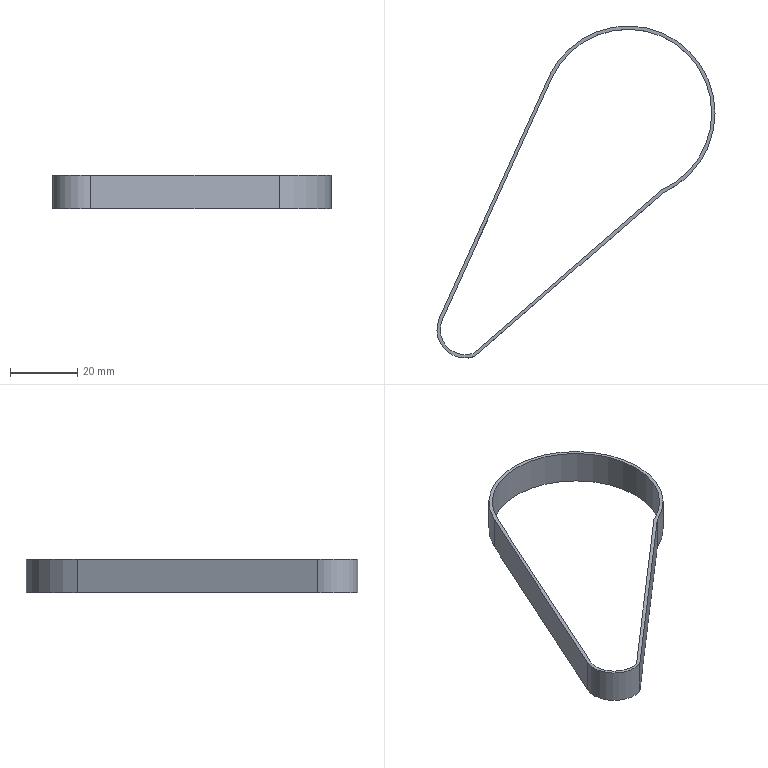Part | SolidWorks | features ExtruThin 1 | 1 solid | 12 faces | box 83.007 x 99.109 x 10 mm | volume 2707 mm3 | cylinder 6 | plane 6 | commonest cylinder face diameters 50 x2 52 x2 15 x1 17 x1
STEP:
#1=CARTESIAN_POINT('',(13.626,44.609,-10.));
#2=VERTEX_POINT('',#1);
#3=CARTESIAN_POINT('',(-34.143,54.932,-10.));
#4=VERTEX_POINT('',#3);
#5=CARTESIAN_POINT('',(-11.374,44.609,-10.));
#6=DIRECTION('',(0.,0.,1.));
#7=DIRECTION('',(1.,0.,0.));
#8=AXIS2_PLACEMENT_3D('',#5,#6,#7);
#9=CIRCLE('',#8,25.);
#10=EDGE_CURVE('',#2,#4,#9,.T.);
#11=ORIENTED_EDGE('',*,*,#10,.F.);
#12=CARTESIAN_POINT('',(13.626,44.609,0.));
#13=VERTEX_POINT('',#12);
#14=CARTESIAN_POINT('',(13.626,44.609,-10.));
#15=DIRECTION('',(0.,0.,1.));
#16=VECTOR('',#15,1000.);
#17=LINE('',#14,#16);
#18=EDGE_CURVE('',#2,#13,#17,.T.);
#19=ORIENTED_EDGE('',*,*,#18,.T.);
#20=CARTESIAN_POINT('',(-34.143,54.932,0.));
#21=VERTEX_POINT('',#20);
#22=CARTESIAN_POINT('',(-11.374,44.609,0.));
#23=DIRECTION('',(0.,0.,1.));
#24=DIRECTION('',(1.,0.,0.));
#25=AXIS2_PLACEMENT_3D('',#22,#23,#24);
#26=CIRCLE('',#25,25.);
#27=EDGE_CURVE('',#13,#21,#26,.T.);
#28=ORIENTED_EDGE('',*,*,#27,.T.);
#29=CARTESIAN_POINT('',(-34.143,54.932,-10.));
#30=DIRECTION('',(0.,0.,1.));
#31=VECTOR('',#30,1000.);
#32=LINE('',#29,#31);
#33=EDGE_CURVE('',#4,#21,#32,.T.);
#34=ORIENTED_EDGE('',*,*,#33,.F.);
#35=EDGE_LOOP('',(#11,#19,#28,#34));
#36=FACE_OUTER_BOUND('',#35,.T.);
#37=CARTESIAN_POINT('',(-11.374,44.609,-10.));
#38=DIRECTION('',(0.,0.,1.));
#39=DIRECTION('',(1.,0.,0.));
#40=AXIS2_PLACEMENT_3D('',#37,#38,#39);
#41=CYLINDRICAL_SURFACE('',#40,25.);
#42=ADVANCED_FACE('',(#36),#41,.F.);
#43=CARTESIAN_POINT('',(-0.8671,20.826,-10.));
#44=VERTEX_POINT('',#43);
#45=CARTESIAN_POINT('',(14.626,44.609,-10.));
#46=VERTEX_POINT('',#45);
#47=CARTESIAN_POINT('',(-11.374,44.609,-10.));
#48=DIRECTION('',(0.,0.,1.));
#49=DIRECTION('',(1.,0.,0.));
#50=AXIS2_PLACEMENT_3D('',#47,#48,#49);
#51=CIRCLE('',#50,26.);
#52=EDGE_CURVE('',#44,#46,#51,.T.);
#53=ORIENTED_EDGE('',*,*,#52,.T.);
#54=CARTESIAN_POINT('',(14.626,44.609,0.));
#55=VERTEX_POINT('',#54);
#56=CARTESIAN_POINT('',(14.626,44.609,-10.));
#57=DIRECTION('',(0.,0.,1.));
#58=VECTOR('',#57,1000.);
#59=LINE('',#56,#58);
#60=EDGE_CURVE('',#46,#55,#59,.T.);
#61=ORIENTED_EDGE('',*,*,#60,.T.);
#62=CARTESIAN_POINT('',(-0.8671,20.826,0.));
#63=VERTEX_POINT('',#62);
#64=CARTESIAN_POINT('',(-11.374,44.609,0.));
#65=DIRECTION('',(0.,0.,1.));
#66=DIRECTION('',(1.,0.,0.));
#67=AXIS2_PLACEMENT_3D('',#64,#65,#66);
#68=CIRCLE('',#67,26.);
#69=EDGE_CURVE('',#63,#55,#68,.T.);
#70=ORIENTED_EDGE('',*,*,#69,.F.);
#71=CARTESIAN_POINT('',(-0.8671,20.826,-10.));
#72=DIRECTION('',(0.,0.,1.));
#73=VECTOR('',#72,1000.);
#74=LINE('',#71,#73);
#75=EDGE_CURVE('',#44,#63,#74,.T.);
#76=ORIENTED_EDGE('',*,*,#75,.F.);
#77=EDGE_LOOP('',(#53,#61,#70,#76));
#78=FACE_OUTER_BOUND('',#77,.T.);
#79=CARTESIAN_POINT('',(-11.374,44.609,-10.));
#80=DIRECTION('',(0.,0.,1.));
#81=DIRECTION('',(1.,0.,0.));
#82=AXIS2_PLACEMENT_3D('',#79,#80,#81);
#83=CYLINDRICAL_SURFACE('',#82,26.);
#84=ADVANCED_FACE('',(#78),#83,.T.);
#85=CARTESIAN_POINT('',(-67.622,-16.49,0.));
#86=VERTEX_POINT('',#85);
#87=CARTESIAN_POINT('',(-57.067,-28.021,0.));
#88=VERTEX_POINT('',#87);
#89=CARTESIAN_POINT('',(-59.88,-20.,0.));
#90=DIRECTION('',(0.,0.,1.));
#91=DIRECTION('',(1.,0.,0.));
#92=AXIS2_PLACEMENT_3D('',#89,#90,#91);
#93=CIRCLE('',#92,8.5);
#94=EDGE_CURVE('',#86,#88,#93,.T.);
#95=ORIENTED_EDGE('',*,*,#94,.F.);
#96=CARTESIAN_POINT('',(-67.622,-16.49,-10.));
#97=VERTEX_POINT('',#96);
#98=CARTESIAN_POINT('',(-67.622,-16.49,-10.));
#99=DIRECTION('',(0.,0.,1.));
#100=VECTOR('',#99,1000.);
#101=LINE('',#98,#100);
#102=EDGE_CURVE('',#97,#86,#101,.T.);
#103=ORIENTED_EDGE('',*,*,#102,.F.);
#104=CARTESIAN_POINT('',(-57.067,-28.021,-10.));
#105=VERTEX_POINT('',#104);
#106=CARTESIAN_POINT('',(-59.88,-20.,-10.));
#107=DIRECTION('',(0.,0.,1.));
#108=DIRECTION('',(1.,0.,0.));
#109=AXIS2_PLACEMENT_3D('',#106,#107,#108);
#110=CIRCLE('',#109,8.5);
#111=EDGE_CURVE('',#97,#105,#110,.T.);
#112=ORIENTED_EDGE('',*,*,#111,.T.);
#113=CARTESIAN_POINT('',(-57.067,-28.021,-10.));
#114=DIRECTION('',(0.,0.,1.));
#115=VECTOR('',#114,1000.);
#116=LINE('',#113,#115);
#117=EDGE_CURVE('',#105,#88,#116,.T.);
#118=ORIENTED_EDGE('',*,*,#117,.T.);
#119=EDGE_LOOP('',(#95,#103,#112,#118));
#120=FACE_OUTER_BOUND('',#119,.T.);
#121=CARTESIAN_POINT('',(-59.88,-20.,-10.));
#122=DIRECTION('',(0.,0.,1.));
#123=DIRECTION('',(1.,0.,0.));
#124=AXIS2_PLACEMENT_3D('',#121,#122,#123);
#125=CYLINDRICAL_SURFACE('',#124,8.5);
#126=ADVANCED_FACE('',(#120),#125,.T.);
#127=CARTESIAN_POINT('',(-35.053,55.345,0.));
#128=VERTEX_POINT('',#127);
#129=CARTESIAN_POINT('',(-67.622,-16.49,0.));
#130=DIRECTION('',(-0.4129,-0.9108,0.));
#131=VECTOR('',#130,1000.);
#132=LINE('',#129,#131);
#133=EDGE_CURVE('',#128,#86,#132,.T.);
#134=ORIENTED_EDGE('',*,*,#133,.F.);
#135=CARTESIAN_POINT('',(-35.053,55.345,-10.));
#136=VERTEX_POINT('',#135);
#137=CARTESIAN_POINT('',(-35.053,55.345,-10.));
#138=DIRECTION('',(0.,0.,1.));
#139=VECTOR('',#138,1000.);
#140=LINE('',#137,#139);
#141=EDGE_CURVE('',#136,#128,#140,.T.);
#142=ORIENTED_EDGE('',*,*,#141,.F.);
#143=CARTESIAN_POINT('',(-67.622,-16.49,-10.));
#144=DIRECTION('',(-0.4129,-0.9108,0.));
#145=VECTOR('',#144,1000.);
#146=LINE('',#143,#145);
#147=EDGE_CURVE('',#136,#97,#146,.T.);
#148=ORIENTED_EDGE('',*,*,#147,.T.);
#149=ORIENTED_EDGE('',*,*,#102,.T.);
#150=EDGE_LOOP('',(#134,#142,#148,#149));
#151=FACE_OUTER_BOUND('',#150,.T.);
#152=CARTESIAN_POINT('',(-67.622,-16.49,-10.));
#153=DIRECTION('',(-0.9108,0.4129,0.));
#154=DIRECTION('',(-0.4129,-0.9108,0.));
#155=AXIS2_PLACEMENT_3D('',#152,#153,#154);
#156=PLANE('',#155);
#157=ADVANCED_FACE('',(#151),#156,.T.);
#158=ORIENTED_EDGE('',*,*,#60,.F.);
#159=CARTESIAN_POINT('',(-11.374,44.609,-10.));
#160=DIRECTION('',(0.,0.,1.));
#161=DIRECTION('',(1.,0.,0.));
#162=AXIS2_PLACEMENT_3D('',#159,#160,#161);
#163=CIRCLE('',#162,26.);
#164=EDGE_CURVE('',#46,#136,#163,.T.);
#165=ORIENTED_EDGE('',*,*,#164,.T.);
#166=ORIENTED_EDGE('',*,*,#141,.T.);
#167=CARTESIAN_POINT('',(-11.374,44.609,0.));
#168=DIRECTION('',(0.,0.,1.));
#169=DIRECTION('',(1.,0.,0.));
#170=AXIS2_PLACEMENT_3D('',#167,#168,#169);
#171=CIRCLE('',#170,26.);
#172=EDGE_CURVE('',#55,#128,#171,.T.);
#173=ORIENTED_EDGE('',*,*,#172,.F.);
#174=EDGE_LOOP('',(#158,#165,#166,#173));
#175=FACE_OUTER_BOUND('',#174,.T.);
#176=CARTESIAN_POINT('',(-11.374,44.609,-10.));
#177=DIRECTION('',(0.,0.,1.));
#178=DIRECTION('',(1.,0.,0.));
#179=AXIS2_PLACEMENT_3D('',#176,#177,#178);
#180=CYLINDRICAL_SURFACE('',#179,26.);
#181=ADVANCED_FACE('',(#175),#180,.T.);
#182=CARTESIAN_POINT('',(-56.918,-27.891,0.));
#183=DIRECTION('',(0.7548,0.656,0.));
#184=VECTOR('',#183,1000.);
#185=LINE('',#182,#184);
#186=EDGE_CURVE('',#88,#63,#185,.T.);
#187=ORIENTED_EDGE('',*,*,#186,.F.);
#188=ORIENTED_EDGE('',*,*,#117,.F.);
#189=CARTESIAN_POINT('',(-56.918,-27.891,-10.));
#190=DIRECTION('',(0.7548,0.656,0.));
#191=VECTOR('',#190,1000.);
#192=LINE('',#189,#191);
#193=EDGE_CURVE('',#105,#44,#192,.T.);
#194=ORIENTED_EDGE('',*,*,#193,.T.);
#195=ORIENTED_EDGE('',*,*,#75,.T.);
#196=EDGE_LOOP('',(#187,#188,#194,#195));
#197=FACE_OUTER_BOUND('',#196,.T.);
#198=CARTESIAN_POINT('',(-56.918,-27.891,-10.));
#199=DIRECTION('',(0.656,-0.7548,0.));
#200=DIRECTION('',(0.7548,0.656,0.));
#201=AXIS2_PLACEMENT_3D('',#198,#199,#200);
#202=PLANE('',#201);
#203=ADVANCED_FACE('',(#197),#202,.T.);
#204=CARTESIAN_POINT('',(-66.711,-16.903,-10.));
#205=VERTEX_POINT('',#204);
#206=CARTESIAN_POINT('',(-66.711,-16.903,-10.));
#207=DIRECTION('',(-0.4129,-0.9108,0.));
#208=VECTOR('',#207,1000.);
#209=LINE('',#206,#208);
#210=EDGE_CURVE('',#4,#205,#209,.T.);
#211=ORIENTED_EDGE('',*,*,#210,.T.);
#212=CARTESIAN_POINT('',(-57.574,-27.137,-10.));
#213=VERTEX_POINT('',#212);
#214=CARTESIAN_POINT('',(-59.88,-20.,-10.));
#215=DIRECTION('',(0.,0.,1.));
#216=DIRECTION('',(1.,0.,0.));
#217=AXIS2_PLACEMENT_3D('',#214,#215,#216);
#218=CIRCLE('',#217,7.5);
#219=EDGE_CURVE('',#205,#213,#218,.T.);
#220=ORIENTED_EDGE('',*,*,#219,.T.);
#221=CARTESIAN_POINT('',(-1.408,21.681,-10.));
#222=VERTEX_POINT('',#221);
#223=CARTESIAN_POINT('',(-57.574,-27.137,-10.));
#224=DIRECTION('',(0.7548,0.656,0.));
#225=VECTOR('',#224,1000.);
#226=LINE('',#223,#225);
#227=EDGE_CURVE('',#213,#222,#226,.T.);
#228=ORIENTED_EDGE('',*,*,#227,.T.);
#229=CARTESIAN_POINT('',(-11.374,44.609,-10.));
#230=DIRECTION('',(0.,0.,1.));
#231=DIRECTION('',(1.,0.,0.));
#232=AXIS2_PLACEMENT_3D('',#229,#230,#231);
#233=CIRCLE('',#232,25.);
#234=EDGE_CURVE('',#222,#2,#233,.T.);
#235=ORIENTED_EDGE('',*,*,#234,.T.);
#236=ORIENTED_EDGE('',*,*,#10,.T.);
#237=EDGE_LOOP('',(#211,#220,#228,#235,#236));
#238=FACE_BOUND('',#237,.T.);
#239=ORIENTED_EDGE('',*,*,#111,.F.);
#240=ORIENTED_EDGE('',*,*,#147,.F.);
#241=ORIENTED_EDGE('',*,*,#164,.F.);
#242=ORIENTED_EDGE('',*,*,#52,.F.);
#243=ORIENTED_EDGE('',*,*,#193,.F.);
#244=EDGE_LOOP('',(#239,#240,#241,#242,#243));
#245=FACE_OUTER_BOUND('',#244,.T.);
#246=CARTESIAN_POINT('',(-59.88,-20.,-10.));
#247=DIRECTION('',(0.,0.,1.));
#248=DIRECTION('',(1.,0.,0.));
#249=AXIS2_PLACEMENT_3D('',#246,#247,#248);
#250=PLANE('',#249);
#251=ADVANCED_FACE('',(#238,#245),#250,.F.);
#252=CARTESIAN_POINT('',(-66.711,-16.903,0.));
#253=VERTEX_POINT('',#252);
#254=CARTESIAN_POINT('',(-57.574,-27.137,0.));
#255=VERTEX_POINT('',#254);
#256=CARTESIAN_POINT('',(-59.88,-20.,0.));
#257=DIRECTION('',(0.,0.,1.));
#258=DIRECTION('',(1.,0.,0.));
#259=AXIS2_PLACEMENT_3D('',#256,#257,#258);
#260=CIRCLE('',#259,7.5);
#261=EDGE_CURVE('',#253,#255,#260,.T.);
#262=ORIENTED_EDGE('',*,*,#261,.F.);
#263=CARTESIAN_POINT('',(-66.711,-16.903,0.));
#264=DIRECTION('',(-0.4129,-0.9108,0.));
#265=VECTOR('',#264,1000.);
#266=LINE('',#263,#265);
#267=EDGE_CURVE('',#21,#253,#266,.T.);
#268=ORIENTED_EDGE('',*,*,#267,.F.);
#269=ORIENTED_EDGE('',*,*,#27,.F.);
#270=CARTESIAN_POINT('',(-1.408,21.681,0.));
#271=VERTEX_POINT('',#270);
#272=CARTESIAN_POINT('',(-11.374,44.609,0.));
#273=DIRECTION('',(0.,0.,1.));
#274=DIRECTION('',(1.,0.,0.));
#275=AXIS2_PLACEMENT_3D('',#272,#273,#274);
#276=CIRCLE('',#275,25.);
#277=EDGE_CURVE('',#271,#13,#276,.T.);
#278=ORIENTED_EDGE('',*,*,#277,.F.);
#279=CARTESIAN_POINT('',(-57.574,-27.137,0.));
#280=DIRECTION('',(0.7548,0.656,0.));
#281=VECTOR('',#280,1000.);
#282=LINE('',#279,#281);
#283=EDGE_CURVE('',#255,#271,#282,.T.);
#284=ORIENTED_EDGE('',*,*,#283,.F.);
#285=EDGE_LOOP('',(#262,#268,#269,#278,#284));
#286=FACE_BOUND('',#285,.T.);
#287=ORIENTED_EDGE('',*,*,#94,.T.);
#288=ORIENTED_EDGE('',*,*,#186,.T.);
#289=ORIENTED_EDGE('',*,*,#69,.T.);
#290=ORIENTED_EDGE('',*,*,#172,.T.);
#291=ORIENTED_EDGE('',*,*,#133,.T.);
#292=EDGE_LOOP('',(#287,#288,#289,#290,#291));
#293=FACE_OUTER_BOUND('',#292,.T.);
#294=CARTESIAN_POINT('',(-59.88,-20.,0.));
#295=DIRECTION('',(0.,0.,1.));
#296=DIRECTION('',(1.,0.,0.));
#297=AXIS2_PLACEMENT_3D('',#294,#295,#296);
#298=PLANE('',#297);
#299=ADVANCED_FACE('',(#286,#293),#298,.T.);
#300=ORIENTED_EDGE('',*,*,#261,.T.);
#301=CARTESIAN_POINT('',(-57.574,-27.137,-10.));
#302=DIRECTION('',(0.,0.,1.));
#303=VECTOR('',#302,1000.);
#304=LINE('',#301,#303);
#305=EDGE_CURVE('',#213,#255,#304,.T.);
#306=ORIENTED_EDGE('',*,*,#305,.F.);
#307=ORIENTED_EDGE('',*,*,#219,.F.);
#308=CARTESIAN_POINT('',(-66.711,-16.903,-10.));
#309=DIRECTION('',(0.,0.,1.));
#310=VECTOR('',#309,1000.);
#311=LINE('',#308,#310);
#312=EDGE_CURVE('',#205,#253,#311,.T.);
#313=ORIENTED_EDGE('',*,*,#312,.T.);
#314=EDGE_LOOP('',(#300,#306,#307,#313));
#315=FACE_OUTER_BOUND('',#314,.T.);
#316=CARTESIAN_POINT('',(-59.88,-20.,-10.));
#317=DIRECTION('',(0.,0.,1.));
#318=DIRECTION('',(1.,0.,0.));
#319=AXIS2_PLACEMENT_3D('',#316,#317,#318);
#320=CYLINDRICAL_SURFACE('',#319,7.5);
#321=ADVANCED_FACE('',(#315),#320,.F.);
#322=ORIENTED_EDGE('',*,*,#267,.T.);
#323=ORIENTED_EDGE('',*,*,#312,.F.);
#324=ORIENTED_EDGE('',*,*,#210,.F.);
#325=ORIENTED_EDGE('',*,*,#33,.T.);
#326=EDGE_LOOP('',(#322,#323,#324,#325));
#327=FACE_OUTER_BOUND('',#326,.T.);
#328=CARTESIAN_POINT('',(-66.711,-16.903,-10.));
#329=DIRECTION('',(-0.9108,0.4129,0.));
#330=DIRECTION('',(-0.4129,-0.9108,0.));
#331=AXIS2_PLACEMENT_3D('',#328,#329,#330);
#332=PLANE('',#331);
#333=ADVANCED_FACE('',(#327),#332,.F.);
#334=ORIENTED_EDGE('',*,*,#18,.F.);
#335=ORIENTED_EDGE('',*,*,#234,.F.);
#336=CARTESIAN_POINT('',(-1.408,21.681,-10.));
#337=DIRECTION('',(0.,0.,1.));
#338=VECTOR('',#337,1000.);
#339=LINE('',#336,#338);
#340=EDGE_CURVE('',#222,#271,#339,.T.);
#341=ORIENTED_EDGE('',*,*,#340,.T.);
#342=ORIENTED_EDGE('',*,*,#277,.T.);
#343=EDGE_LOOP('',(#334,#335,#341,#342));
#344=FACE_OUTER_BOUND('',#343,.T.);
#345=CARTESIAN_POINT('',(-11.374,44.609,-10.));
#346=DIRECTION('',(0.,0.,1.));
#347=DIRECTION('',(1.,0.,0.));
#348=AXIS2_PLACEMENT_3D('',#345,#346,#347);
#349=CYLINDRICAL_SURFACE('',#348,25.);
#350=ADVANCED_FACE('',(#344),#349,.F.);
#351=ORIENTED_EDGE('',*,*,#283,.T.);
#352=ORIENTED_EDGE('',*,*,#340,.F.);
#353=ORIENTED_EDGE('',*,*,#227,.F.);
#354=ORIENTED_EDGE('',*,*,#305,.T.);
#355=EDGE_LOOP('',(#351,#352,#353,#354));
#356=FACE_OUTER_BOUND('',#355,.T.);
#357=CARTESIAN_POINT('',(-57.574,-27.137,-10.));
#358=DIRECTION('',(0.656,-0.7548,0.));
#359=DIRECTION('',(0.7548,0.656,0.));
#360=AXIS2_PLACEMENT_3D('',#357,#358,#359);
#361=PLANE('',#360);
#362=ADVANCED_FACE('',(#356),#361,.F.);
#363=CLOSED_SHELL('',(#42,#84,#126,#157,#181,#203,#251,#299,#321,#333,#350,#362));
#364=MANIFOLD_SOLID_BREP('',#363);
#365=CARTESIAN_POINT('',(0.,0.,0.));
#366=DIRECTION('',(0.,0.,1.));
#367=DIRECTION('',(1.,0.,0.));
#368=AXIS2_PLACEMENT_3D('',#365,#366,#367);
#369=(LENGTH_UNIT()NAMED_UNIT(*)SI_UNIT(.MILLI.,.METRE.));
#370=UNCERTAINTY_MEASURE_WITH_UNIT(LENGTH_MEASURE(0.00001),#369,'','');
#371=(NAMED_UNIT(*)PLANE_ANGLE_UNIT()SI_UNIT($,.RADIAN.));
#372=(NAMED_UNIT(*)SI_UNIT($,.STERADIAN.)SOLID_ANGLE_UNIT());
#373=(GEOMETRIC_REPRESENTATION_CONTEXT(3)GLOBAL_UNCERTAINTY_ASSIGNED_CONTEXT((#370))GLOBAL_UNIT_ASSIGNED_CONTEXT((#369,#371,#372))REPRESENTATION_CONTEXT('',''));
#374=ADVANCED_BREP_SHAPE_REPRESENTATION('',(#364,#368),#373);